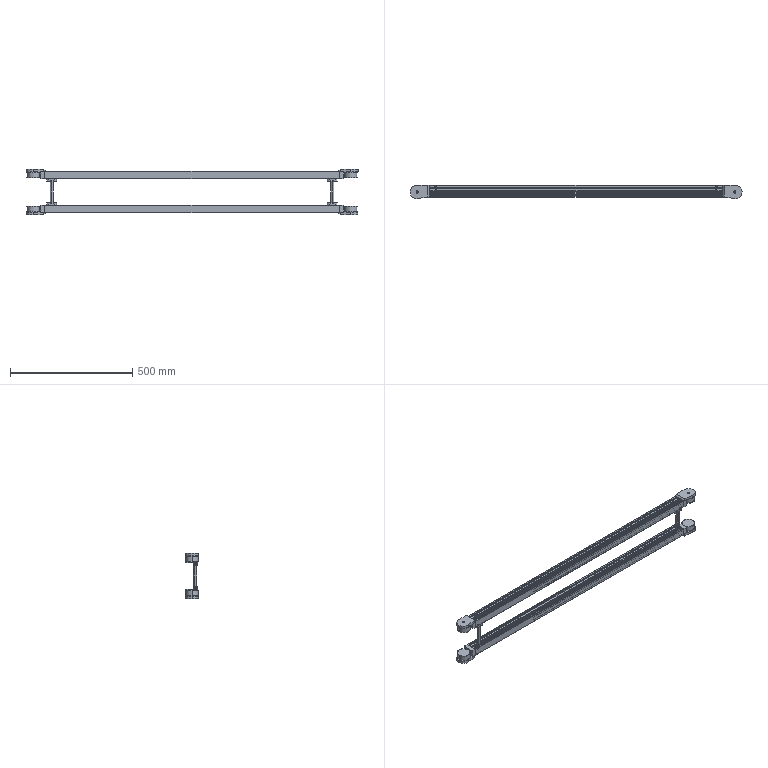Part | STEP file | Guide wheel mechanism revised.sldasm-Part-327 | 1 solid | 921 faces | box 1360 x 54 x 186 mm | volume 2730311 mm3 | plane 703 | cylinder 194 | cone 24 | commonest cylinder face diameters 12.2 x32 54 x22 6 x16 6.4 x16 7.2 x16 10 x16